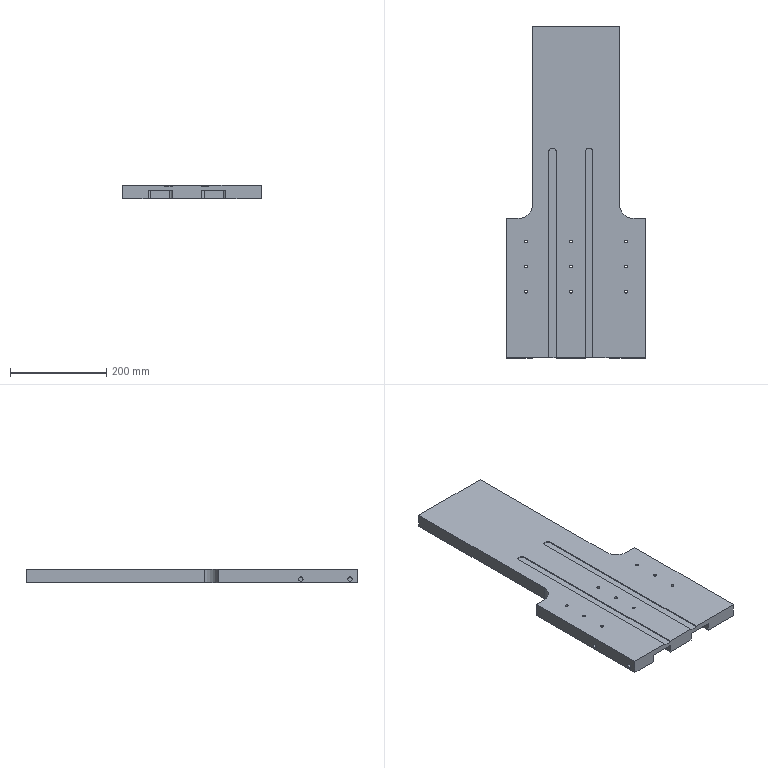Part | Creo | features CURVE 9, CUT 5, PROTRUSION 4, DATUM PLANE 3, ROUND 3, COORDINATE SYSTEM 1 | 1 solid | 89 faces | box 289.25 x 690 x 28 mm | volume 4080751 mm3 | cylinder 54 | plane 35 | commonest cylinder face diameters 6 x18 10.049 x18 9 x8 10 x8 60 x2